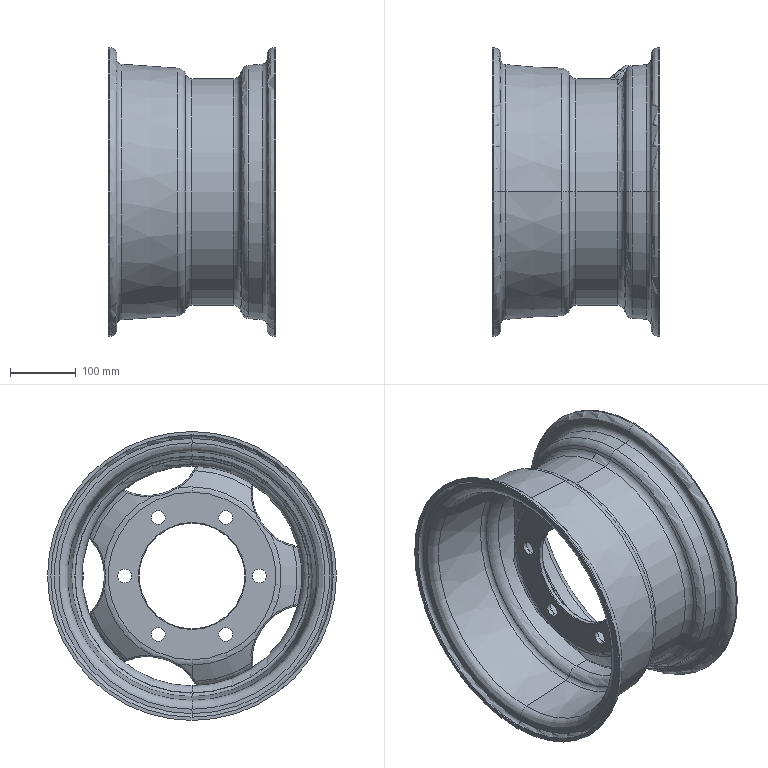Part | STEP file | FELGA_9.00x15.3V11 | 1 solid | 295 faces | box 254.399 x 439.355 x 439.355 mm | volume 2312376 mm3 | spline 108 | torus 65 | cone 50 | cylinder 45 | plane 27 | commonest cylinder face diameters 21 x12 36 x6 320.56 x5 8 x4 429.355 x4 439.355 x4